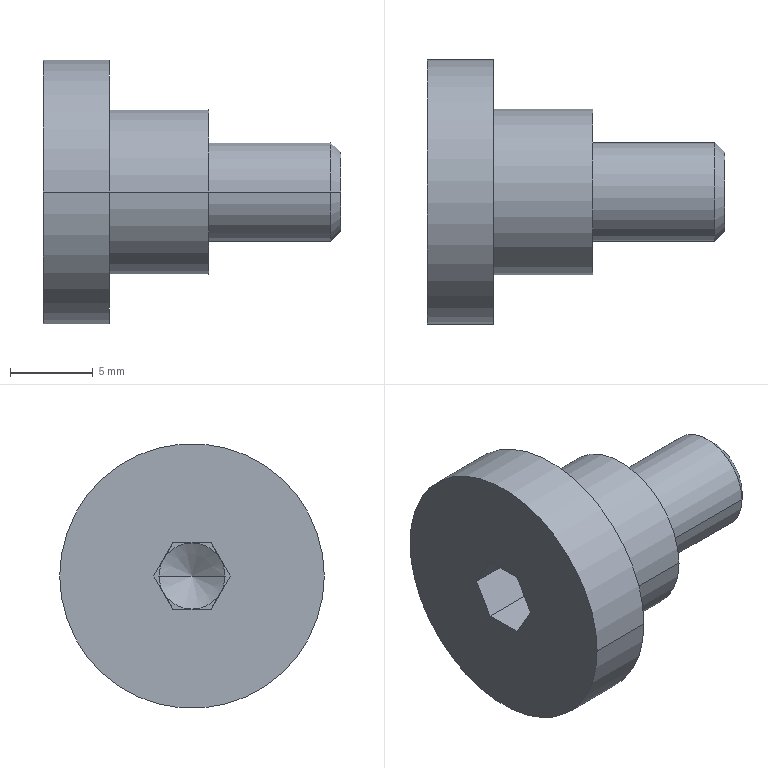Part | STEP file | pivot pin bolt DBS6-6-8 | 1 solid | 26 faces | box 18 x 16 x 16 mm | volume 1445 mm3 | plane 16 | cylinder 6 | cone 4 | commonest cylinder face diameters 6 x2 10 x2 16 x2